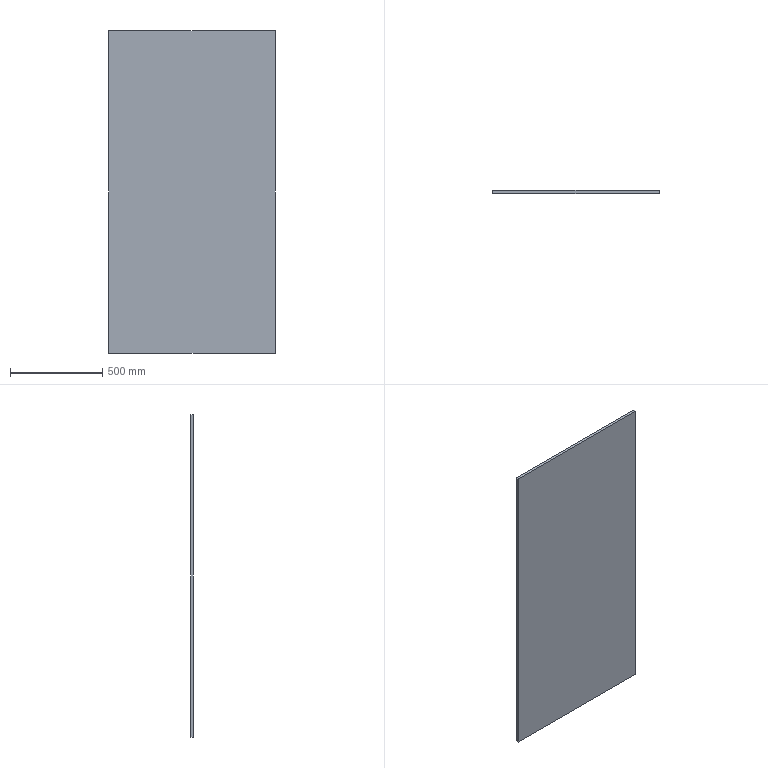Part | SolidWorks | features Extrusion 1 | 1 solid | 6 faces | box 903 x 15 x 1750 mm | volume 23703750 mm3 | plane 6
STEP:
#1=CARTESIAN_POINT('',(0.,0.,0.));
#2=VERTEX_POINT('',#1);
#3=CARTESIAN_POINT('',(0.,0.,1750.));
#4=VERTEX_POINT('',#3);
#5=CARTESIAN_POINT('',(0.,0.,1750.));
#6=DIRECTION('',(0.,0.,1.));
#7=VECTOR('',#6,1000.);
#8=LINE('',#5,#7);
#9=EDGE_CURVE('',#2,#4,#8,.T.);
#10=ORIENTED_EDGE('',*,*,#9,.T.);
#11=CARTESIAN_POINT('',(0.,15.,1750.));
#12=VERTEX_POINT('',#11);
#13=CARTESIAN_POINT('',(0.,15.,1750.));
#14=DIRECTION('',(0.,-1.,0.));
#15=VECTOR('',#14,1000.);
#16=LINE('',#13,#15);
#17=EDGE_CURVE('',#12,#4,#16,.T.);
#18=ORIENTED_EDGE('',*,*,#17,.F.);
#19=CARTESIAN_POINT('',(0.,15.,0.));
#20=VERTEX_POINT('',#19);
#21=CARTESIAN_POINT('',(0.,15.,1750.));
#22=DIRECTION('',(0.,0.,1.));
#23=VECTOR('',#22,1000.);
#24=LINE('',#21,#23);
#25=EDGE_CURVE('',#20,#12,#24,.T.);
#26=ORIENTED_EDGE('',*,*,#25,.F.);
#27=CARTESIAN_POINT('',(0.,15.,0.));
#28=DIRECTION('',(0.,-1.,0.));
#29=VECTOR('',#28,1000.);
#30=LINE('',#27,#29);
#31=EDGE_CURVE('',#20,#2,#30,.T.);
#32=ORIENTED_EDGE('',*,*,#31,.T.);
#33=EDGE_LOOP('',(#10,#18,#26,#32));
#34=FACE_OUTER_BOUND('',#33,.T.);
#35=CARTESIAN_POINT('',(0.,15.,1750.));
#36=DIRECTION('',(1.,0.,0.));
#37=DIRECTION('',(0.,0.,-1.));
#38=AXIS2_PLACEMENT_3D('',#35,#36,#37);
#39=PLANE('',#38);
#40=ADVANCED_FACE('',(#34),#39,.F.);
#41=CARTESIAN_POINT('',(903.,0.,1750.));
#42=VERTEX_POINT('',#41);
#43=CARTESIAN_POINT('',(903.,0.,1750.));
#44=DIRECTION('',(1.,0.,0.));
#45=VECTOR('',#44,1000.);
#46=LINE('',#43,#45);
#47=EDGE_CURVE('',#4,#42,#46,.T.);
#48=ORIENTED_EDGE('',*,*,#47,.T.);
#49=CARTESIAN_POINT('',(903.,15.,1750.));
#50=VERTEX_POINT('',#49);
#51=CARTESIAN_POINT('',(903.,15.,1750.));
#52=DIRECTION('',(0.,-1.,0.));
#53=VECTOR('',#52,1000.);
#54=LINE('',#51,#53);
#55=EDGE_CURVE('',#50,#42,#54,.T.);
#56=ORIENTED_EDGE('',*,*,#55,.F.);
#57=CARTESIAN_POINT('',(903.,15.,1750.));
#58=DIRECTION('',(1.,0.,0.));
#59=VECTOR('',#58,1000.);
#60=LINE('',#57,#59);
#61=EDGE_CURVE('',#12,#50,#60,.T.);
#62=ORIENTED_EDGE('',*,*,#61,.F.);
#63=ORIENTED_EDGE('',*,*,#17,.T.);
#64=EDGE_LOOP('',(#48,#56,#62,#63));
#65=FACE_OUTER_BOUND('',#64,.T.);
#66=CARTESIAN_POINT('',(903.,15.,1750.));
#67=DIRECTION('',(0.,0.,-1.));
#68=DIRECTION('',(-1.,0.,0.));
#69=AXIS2_PLACEMENT_3D('',#66,#67,#68);
#70=PLANE('',#69);
#71=ADVANCED_FACE('',(#65),#70,.F.);
#72=CARTESIAN_POINT('',(903.,0.,0.));
#73=VERTEX_POINT('',#72);
#74=CARTESIAN_POINT('',(903.,0.,0.));
#75=DIRECTION('',(0.,0.,-1.));
#76=VECTOR('',#75,1000.);
#77=LINE('',#74,#76);
#78=EDGE_CURVE('',#42,#73,#77,.T.);
#79=ORIENTED_EDGE('',*,*,#78,.T.);
#80=CARTESIAN_POINT('',(903.,15.,0.));
#81=VERTEX_POINT('',#80);
#82=CARTESIAN_POINT('',(903.,15.,0.));
#83=DIRECTION('',(0.,-1.,0.));
#84=VECTOR('',#83,1000.);
#85=LINE('',#82,#84);
#86=EDGE_CURVE('',#81,#73,#85,.T.);
#87=ORIENTED_EDGE('',*,*,#86,.F.);
#88=CARTESIAN_POINT('',(903.,15.,0.));
#89=DIRECTION('',(0.,0.,-1.));
#90=VECTOR('',#89,1000.);
#91=LINE('',#88,#90);
#92=EDGE_CURVE('',#50,#81,#91,.T.);
#93=ORIENTED_EDGE('',*,*,#92,.F.);
#94=ORIENTED_EDGE('',*,*,#55,.T.);
#95=EDGE_LOOP('',(#79,#87,#93,#94));
#96=FACE_OUTER_BOUND('',#95,.T.);
#97=CARTESIAN_POINT('',(903.,15.,0.));
#98=DIRECTION('',(-1.,0.,0.));
#99=DIRECTION('',(0.,0.,1.));
#100=AXIS2_PLACEMENT_3D('',#97,#98,#99);
#101=PLANE('',#100);
#102=ADVANCED_FACE('',(#96),#101,.F.);
#103=CARTESIAN_POINT('',(0.,0.,0.));
#104=DIRECTION('',(-1.,0.,0.));
#105=VECTOR('',#104,1000.);
#106=LINE('',#103,#105);
#107=EDGE_CURVE('',#73,#2,#106,.T.);
#108=ORIENTED_EDGE('',*,*,#107,.T.);
#109=ORIENTED_EDGE('',*,*,#31,.F.);
#110=CARTESIAN_POINT('',(0.,15.,0.));
#111=DIRECTION('',(-1.,0.,0.));
#112=VECTOR('',#111,1000.);
#113=LINE('',#110,#112);
#114=EDGE_CURVE('',#81,#20,#113,.T.);
#115=ORIENTED_EDGE('',*,*,#114,.F.);
#116=ORIENTED_EDGE('',*,*,#86,.T.);
#117=EDGE_LOOP('',(#108,#109,#115,#116));
#118=FACE_OUTER_BOUND('',#117,.T.);
#119=CARTESIAN_POINT('',(0.,15.,0.));
#120=DIRECTION('',(0.,0.,1.));
#121=DIRECTION('',(1.,0.,0.));
#122=AXIS2_PLACEMENT_3D('',#119,#120,#121);
#123=PLANE('',#122);
#124=ADVANCED_FACE('',(#118),#123,.F.);
#125=ORIENTED_EDGE('',*,*,#25,.T.);
#126=ORIENTED_EDGE('',*,*,#61,.T.);
#127=ORIENTED_EDGE('',*,*,#92,.T.);
#128=ORIENTED_EDGE('',*,*,#114,.T.);
#129=EDGE_LOOP('',(#125,#126,#127,#128));
#130=FACE_OUTER_BOUND('',#129,.T.);
#131=CARTESIAN_POINT('',(0.,15.,0.));
#132=DIRECTION('',(0.,-1.,0.));
#133=DIRECTION('',(0.,0.,-1.));
#134=AXIS2_PLACEMENT_3D('',#131,#132,#133);
#135=PLANE('',#134);
#136=ADVANCED_FACE('',(#130),#135,.F.);
#137=ORIENTED_EDGE('',*,*,#9,.F.);
#138=ORIENTED_EDGE('',*,*,#107,.F.);
#139=ORIENTED_EDGE('',*,*,#78,.F.);
#140=ORIENTED_EDGE('',*,*,#47,.F.);
#141=EDGE_LOOP('',(#137,#138,#139,#140));
#142=FACE_OUTER_BOUND('',#141,.T.);
#143=CARTESIAN_POINT('',(0.,0.,0.));
#144=DIRECTION('',(0.,-1.,0.));
#145=DIRECTION('',(0.,0.,-1.));
#146=AXIS2_PLACEMENT_3D('',#143,#144,#145);
#147=PLANE('',#146);
#148=ADVANCED_FACE('',(#142),#147,.T.);
#149=CLOSED_SHELL('',(#40,#71,#102,#124,#136,#148));
#150=MANIFOLD_SOLID_BREP('',#149);
#151=CARTESIAN_POINT('',(0.,0.,0.));
#152=DIRECTION('',(0.,0.,1.));
#153=DIRECTION('',(1.,0.,0.));
#154=AXIS2_PLACEMENT_3D('',#151,#152,#153);
#155=(LENGTH_UNIT()NAMED_UNIT(*)SI_UNIT(.MILLI.,.METRE.));
#156=UNCERTAINTY_MEASURE_WITH_UNIT(LENGTH_MEASURE(0.00001),#155,'','');
#157=(NAMED_UNIT(*)PLANE_ANGLE_UNIT()SI_UNIT($,.RADIAN.));
#158=(NAMED_UNIT(*)SI_UNIT($,.STERADIAN.)SOLID_ANGLE_UNIT());
#159=(GEOMETRIC_REPRESENTATION_CONTEXT(3)GLOBAL_UNCERTAINTY_ASSIGNED_CONTEXT((#156))GLOBAL_UNIT_ASSIGNED_CONTEXT((#155,#157,#158))REPRESENTATION_CONTEXT('',''));
#160=ADVANCED_BREP_SHAPE_REPRESENTATION('',(#150,#154),#159);